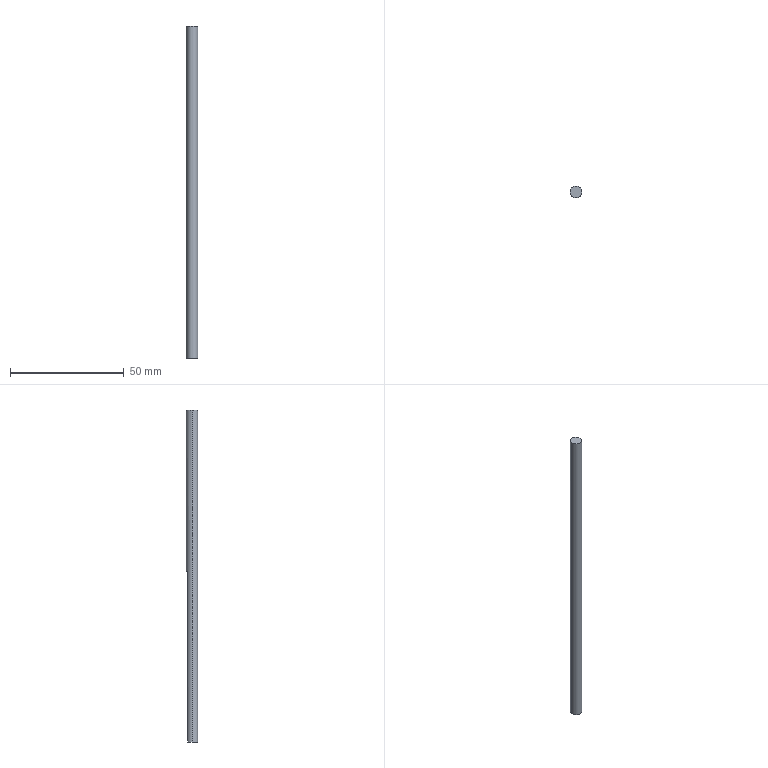Part | SolidWorks | features ICE 2, Extrusion 1 | 1 solid | 6 faces | box 5 x 5 x 146 mm | volume 2741 mm3 | plane 4 | cylinder 2 | commonest cylinder face diameters 5 x2
STEP:
#1=CARTESIAN_POINT('',(2.5,0.,146.));
#2=VERTEX_POINT('',#1);
#3=CARTESIAN_POINT('',(-2.5,0.,146.));
#4=VERTEX_POINT('',#3);
#5=CARTESIAN_POINT('',(0.,0.,146.));
#6=DIRECTION('',(0.,0.,1.));
#7=DIRECTION('',(1.,0.,0.));
#8=AXIS2_PLACEMENT_3D('',#5,#6,#7);
#9=CIRCLE('',#8,2.5);
#10=EDGE_CURVE('',#2,#4,#9,.T.);
#11=ORIENTED_EDGE('',*,*,#10,.F.);
#12=CARTESIAN_POINT('',(2.5,0.,0.));
#13=VERTEX_POINT('',#12);
#14=CARTESIAN_POINT('',(2.5,0.,162.));
#15=DIRECTION('',(0.,0.,-1.));
#16=VECTOR('',#15,1000.);
#17=LINE('',#14,#16);
#18=EDGE_CURVE('',#2,#13,#17,.T.);
#19=ORIENTED_EDGE('',*,*,#18,.T.);
#20=CARTESIAN_POINT('',(1.735,1.8,0.));
#21=VERTEX_POINT('',#20);
#22=CARTESIAN_POINT('',(0.,0.,0.));
#23=DIRECTION('',(0.,0.,1.));
#24=DIRECTION('',(1.,0.,0.));
#25=AXIS2_PLACEMENT_3D('',#22,#23,#24);
#26=CIRCLE('',#25,2.5);
#27=EDGE_CURVE('',#13,#21,#26,.T.);
#28=ORIENTED_EDGE('',*,*,#27,.T.);
#29=CARTESIAN_POINT('',(1.735,1.8,75.));
#30=VERTEX_POINT('',#29);
#31=CARTESIAN_POINT('',(1.735,1.8,75.));
#32=DIRECTION('',(0.,0.,-1.));
#33=VECTOR('',#32,1000.);
#34=LINE('',#31,#33);
#35=EDGE_CURVE('',#30,#21,#34,.T.);
#36=ORIENTED_EDGE('',*,*,#35,.F.);
#37=CARTESIAN_POINT('',(-1.735,1.8,75.));
#38=VERTEX_POINT('',#37);
#39=CARTESIAN_POINT('',(0.,0.,75.));
#40=DIRECTION('',(0.,0.,-1.));
#41=DIRECTION('',(-1.,0.,0.));
#42=AXIS2_PLACEMENT_3D('',#39,#40,#41);
#43=CIRCLE('',#42,2.5);
#44=EDGE_CURVE('',#38,#30,#43,.T.);
#45=ORIENTED_EDGE('',*,*,#44,.F.);
#46=CARTESIAN_POINT('',(-1.735,1.8,0.));
#47=VERTEX_POINT('',#46);
#48=CARTESIAN_POINT('',(-1.735,1.8,75.));
#49=DIRECTION('',(0.,0.,-1.));
#50=VECTOR('',#49,1000.);
#51=LINE('',#48,#50);
#52=EDGE_CURVE('',#38,#47,#51,.T.);
#53=ORIENTED_EDGE('',*,*,#52,.T.);
#54=CARTESIAN_POINT('',(-2.5,0.,0.));
#55=VERTEX_POINT('',#54);
#56=CARTESIAN_POINT('',(0.,0.,0.));
#57=DIRECTION('',(0.,0.,1.));
#58=DIRECTION('',(1.,0.,0.));
#59=AXIS2_PLACEMENT_3D('',#56,#57,#58);
#60=CIRCLE('',#59,2.5);
#61=EDGE_CURVE('',#47,#55,#60,.T.);
#62=ORIENTED_EDGE('',*,*,#61,.T.);
#63=CARTESIAN_POINT('',(-2.5,0.,162.));
#64=DIRECTION('',(0.,0.,-1.));
#65=VECTOR('',#64,1000.);
#66=LINE('',#63,#65);
#67=EDGE_CURVE('',#4,#55,#66,.T.);
#68=ORIENTED_EDGE('',*,*,#67,.F.);
#69=EDGE_LOOP('',(#11,#19,#28,#36,#45,#53,#62,#68));
#70=FACE_OUTER_BOUND('',#69,.T.);
#71=CARTESIAN_POINT('',(0.,0.,162.));
#72=DIRECTION('',(0.,0.,-1.));
#73=DIRECTION('',(-1.,0.,0.));
#74=AXIS2_PLACEMENT_3D('',#71,#72,#73);
#75=CYLINDRICAL_SURFACE('',#74,2.5);
#76=ADVANCED_FACE('',(#70),#75,.T.);
#77=ORIENTED_EDGE('',*,*,#18,.F.);
#78=CARTESIAN_POINT('',(0.,0.,146.));
#79=DIRECTION('',(0.,0.,1.));
#80=DIRECTION('',(1.,0.,0.));
#81=AXIS2_PLACEMENT_3D('',#78,#79,#80);
#82=CIRCLE('',#81,2.5);
#83=EDGE_CURVE('',#4,#2,#82,.T.);
#84=ORIENTED_EDGE('',*,*,#83,.F.);
#85=ORIENTED_EDGE('',*,*,#67,.T.);
#86=CARTESIAN_POINT('',(0.,0.,0.));
#87=DIRECTION('',(0.,0.,1.));
#88=DIRECTION('',(1.,0.,0.));
#89=AXIS2_PLACEMENT_3D('',#86,#87,#88);
#90=CIRCLE('',#89,2.5);
#91=EDGE_CURVE('',#55,#13,#90,.T.);
#92=ORIENTED_EDGE('',*,*,#91,.T.);
#93=EDGE_LOOP('',(#77,#84,#85,#92));
#94=FACE_OUTER_BOUND('',#93,.T.);
#95=CARTESIAN_POINT('',(0.,0.,162.));
#96=DIRECTION('',(0.,0.,-1.));
#97=DIRECTION('',(-1.,0.,0.));
#98=AXIS2_PLACEMENT_3D('',#95,#96,#97);
#99=CYLINDRICAL_SURFACE('',#98,2.5);
#100=ADVANCED_FACE('',(#94),#99,.T.);
#101=ORIENTED_EDGE('',*,*,#61,.F.);
#102=CARTESIAN_POINT('',(0.,1.8,0.));
#103=DIRECTION('',(-1.,0.,0.));
#104=VECTOR('',#103,1000.);
#105=LINE('',#102,#104);
#106=EDGE_CURVE('',#21,#47,#105,.T.);
#107=ORIENTED_EDGE('',*,*,#106,.F.);
#108=ORIENTED_EDGE('',*,*,#27,.F.);
#109=ORIENTED_EDGE('',*,*,#91,.F.);
#110=EDGE_LOOP('',(#101,#107,#108,#109));
#111=FACE_OUTER_BOUND('',#110,.T.);
#112=CARTESIAN_POINT('',(0.,0.,0.));
#113=DIRECTION('',(0.,0.,1.));
#114=DIRECTION('',(1.,0.,0.));
#115=AXIS2_PLACEMENT_3D('',#112,#113,#114);
#116=PLANE('',#115);
#117=ADVANCED_FACE('',(#111),#116,.F.);
#118=ORIENTED_EDGE('',*,*,#106,.T.);
#119=ORIENTED_EDGE('',*,*,#52,.F.);
#120=CARTESIAN_POINT('',(0.,1.8,75.));
#121=DIRECTION('',(-1.,0.,0.));
#122=VECTOR('',#121,1000.);
#123=LINE('',#120,#122);
#124=EDGE_CURVE('',#30,#38,#123,.T.);
#125=ORIENTED_EDGE('',*,*,#124,.F.);
#126=ORIENTED_EDGE('',*,*,#35,.T.);
#127=EDGE_LOOP('',(#118,#119,#125,#126));
#128=FACE_OUTER_BOUND('',#127,.T.);
#129=CARTESIAN_POINT('',(0.,1.8,75.));
#130=DIRECTION('',(0.,-1.,0.));
#131=DIRECTION('',(0.,0.,-1.));
#132=AXIS2_PLACEMENT_3D('',#129,#130,#131);
#133=PLANE('',#132);
#134=ADVANCED_FACE('',(#128),#133,.F.);
#135=ORIENTED_EDGE('',*,*,#124,.T.);
#136=ORIENTED_EDGE('',*,*,#44,.T.);
#137=EDGE_LOOP('',(#135,#136));
#138=FACE_OUTER_BOUND('',#137,.T.);
#139=CARTESIAN_POINT('',(0.,0.,75.));
#140=DIRECTION('',(0.,0.,-1.));
#141=DIRECTION('',(-1.,0.,0.));
#142=AXIS2_PLACEMENT_3D('',#139,#140,#141);
#143=PLANE('',#142);
#144=ADVANCED_FACE('',(#138),#143,.T.);
#145=ORIENTED_EDGE('',*,*,#83,.T.);
#146=ORIENTED_EDGE('',*,*,#10,.T.);
#147=EDGE_LOOP('',(#145,#146));
#148=FACE_OUTER_BOUND('',#147,.T.);
#149=CARTESIAN_POINT('',(0.,0.,146.));
#150=DIRECTION('',(0.,0.,1.));
#151=DIRECTION('',(1.,0.,0.));
#152=AXIS2_PLACEMENT_3D('',#149,#150,#151);
#153=PLANE('',#152);
#154=ADVANCED_FACE('',(#148),#153,.T.);
#155=CLOSED_SHELL('',(#76,#100,#117,#134,#144,#154));
#156=MANIFOLD_SOLID_BREP('',#155);
#157=CARTESIAN_POINT('',(0.,0.,0.));
#158=DIRECTION('',(0.,0.,1.));
#159=DIRECTION('',(1.,0.,0.));
#160=AXIS2_PLACEMENT_3D('',#157,#158,#159);
#161=(LENGTH_UNIT()NAMED_UNIT(*)SI_UNIT(.MILLI.,.METRE.));
#162=UNCERTAINTY_MEASURE_WITH_UNIT(LENGTH_MEASURE(0.00001),#161,'','');
#163=(NAMED_UNIT(*)PLANE_ANGLE_UNIT()SI_UNIT($,.RADIAN.));
#164=(NAMED_UNIT(*)SI_UNIT($,.STERADIAN.)SOLID_ANGLE_UNIT());
#165=(GEOMETRIC_REPRESENTATION_CONTEXT(3)GLOBAL_UNCERTAINTY_ASSIGNED_CONTEXT((#162))GLOBAL_UNIT_ASSIGNED_CONTEXT((#161,#163,#164))REPRESENTATION_CONTEXT('',''));
#166=ADVANCED_BREP_SHAPE_REPRESENTATION('',(#156,#160),#165);